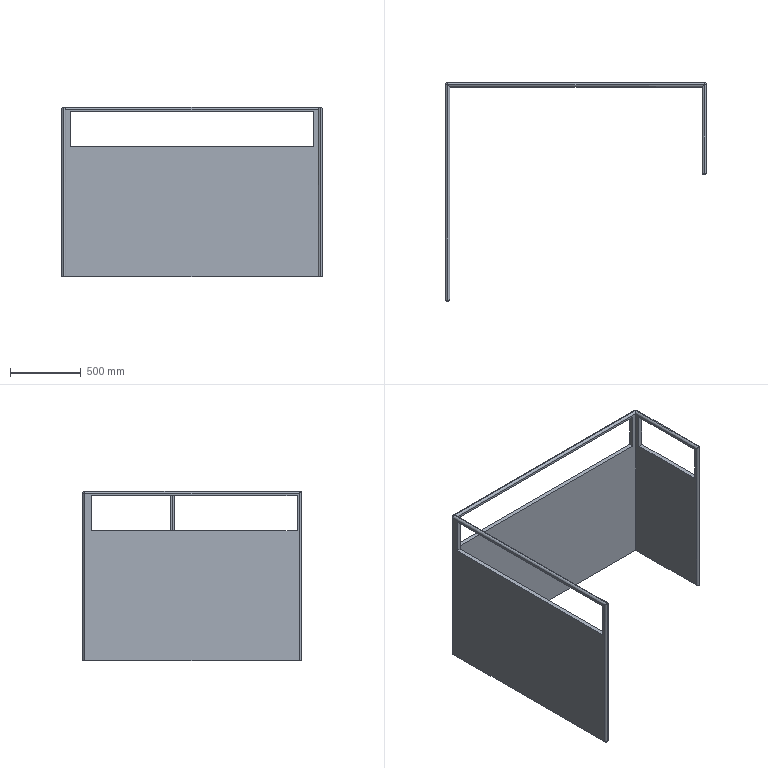Part | SolidWorks | features ICE 3, Extrusion 1, Fillet 1 | 1 solid | 33 faces | box 1850 x 1550 x 1200 mm | volume 114783805 mm3 | plane 19 | cylinder 12 | sphere 2 | commonest cylinder face diameters 30 x12
STEP:
#1=CARTESIAN_POINT('',(30.,30.,1170.));
#2=VERTEX_POINT('',#1);
#3=CARTESIAN_POINT('',(30.,30.,920.));
#4=VERTEX_POINT('',#3);
#5=CARTESIAN_POINT('',(30.,30.,1170.));
#6=DIRECTION('',(0.,0.,-1.));
#7=VECTOR('',#6,1000.);
#8=LINE('',#5,#7);
#9=EDGE_CURVE('',#2,#4,#8,.T.);
#10=ORIENTED_EDGE('',*,*,#9,.F.);
#11=CARTESIAN_POINT('',(30.,1490.,1170.));
#12=VERTEX_POINT('',#11);
#13=CARTESIAN_POINT('',(30.,1490.,1170.));
#14=DIRECTION('',(0.,-1.,0.));
#15=VECTOR('',#14,1000.);
#16=LINE('',#13,#15);
#17=EDGE_CURVE('',#12,#2,#16,.T.);
#18=ORIENTED_EDGE('',*,*,#17,.F.);
#19=CARTESIAN_POINT('',(30.,1490.,920.));
#20=VERTEX_POINT('',#19);
#21=CARTESIAN_POINT('',(30.,1490.,1170.));
#22=DIRECTION('',(0.,0.,1.));
#23=VECTOR('',#22,1000.);
#24=LINE('',#21,#23);
#25=EDGE_CURVE('',#20,#12,#24,.T.);
#26=ORIENTED_EDGE('',*,*,#25,.F.);
#27=CARTESIAN_POINT('',(30.,1490.,920.));
#28=DIRECTION('',(0.,1.,0.));
#29=VECTOR('',#28,1000.);
#30=LINE('',#27,#29);
#31=EDGE_CURVE('',#4,#20,#30,.T.);
#32=ORIENTED_EDGE('',*,*,#31,.F.);
#33=EDGE_LOOP('',(#10,#18,#26,#32));
#34=FACE_BOUND('',#33,.T.);
#35=CARTESIAN_POINT('',(30.,1520.,1185.));
#36=VERTEX_POINT('',#35);
#37=CARTESIAN_POINT('',(30.,15.,1185.));
#38=VERTEX_POINT('',#37);
#39=CARTESIAN_POINT('',(30.,0.,1185.));
#40=DIRECTION('',(0.,-1.,0.));
#41=VECTOR('',#40,1000.);
#42=LINE('',#39,#41);
#43=EDGE_CURVE('',#36,#38,#42,.T.);
#44=ORIENTED_EDGE('',*,*,#43,.T.);
#45=CARTESIAN_POINT('',(30.,15.,0.));
#46=VERTEX_POINT('',#45);
#47=CARTESIAN_POINT('',(30.,15.,1200.));
#48=DIRECTION('',(0.,0.,-1.));
#49=VECTOR('',#48,1000.);
#50=LINE('',#47,#49);
#51=EDGE_CURVE('',#38,#46,#50,.T.);
#52=ORIENTED_EDGE('',*,*,#51,.T.);
#53=CARTESIAN_POINT('',(30.,1520.,0.));
#54=VERTEX_POINT('',#53);
#55=CARTESIAN_POINT('',(30.,0.,0.));
#56=DIRECTION('',(0.,1.,0.));
#57=VECTOR('',#56,1000.);
#58=LINE('',#55,#57);
#59=EDGE_CURVE('',#46,#54,#58,.T.);
#60=ORIENTED_EDGE('',*,*,#59,.T.);
#61=CARTESIAN_POINT('',(30.,1520.,1200.));
#62=DIRECTION('',(0.,0.,-1.));
#63=VECTOR('',#62,1000.);
#64=LINE('',#61,#63);
#65=EDGE_CURVE('',#36,#54,#64,.T.);
#66=ORIENTED_EDGE('',*,*,#65,.F.);
#67=EDGE_LOOP('',(#44,#52,#60,#66));
#68=FACE_OUTER_BOUND('',#67,.T.);
#69=CARTESIAN_POINT('',(30.,0.,1200.));
#70=DIRECTION('',(-1.,0.,0.));
#71=DIRECTION('',(0.,0.,1.));
#72=AXIS2_PLACEMENT_3D('',#69,#70,#71);
#73=PLANE('',#72);
#74=ADVANCED_FACE('',(#34,#68),#73,.F.);
#75=CARTESIAN_POINT('',(60.,1520.,920.));
#76=VERTEX_POINT('',#75);
#77=CARTESIAN_POINT('',(1790.,1520.,920.));
#78=VERTEX_POINT('',#77);
#79=CARTESIAN_POINT('',(60.,1520.,920.));
#80=DIRECTION('',(1.,0.,0.));
#81=VECTOR('',#80,1000.);
#82=LINE('',#79,#81);
#83=EDGE_CURVE('',#76,#78,#82,.T.);
#84=ORIENTED_EDGE('',*,*,#83,.F.);
#85=CARTESIAN_POINT('',(60.,1520.,1170.));
#86=VERTEX_POINT('',#85);
#87=CARTESIAN_POINT('',(60.,1520.,1170.));
#88=DIRECTION('',(0.,0.,-1.));
#89=VECTOR('',#88,1000.);
#90=LINE('',#87,#89);
#91=EDGE_CURVE('',#86,#76,#90,.T.);
#92=ORIENTED_EDGE('',*,*,#91,.F.);
#93=CARTESIAN_POINT('',(1790.,1520.,1170.));
#94=VERTEX_POINT('',#93);
#95=CARTESIAN_POINT('',(60.,1520.,1170.));
#96=DIRECTION('',(-1.,0.,0.));
#97=VECTOR('',#96,1000.);
#98=LINE('',#95,#97);
#99=EDGE_CURVE('',#94,#86,#98,.T.);
#100=ORIENTED_EDGE('',*,*,#99,.F.);
#101=CARTESIAN_POINT('',(1790.,1520.,1170.));
#102=DIRECTION('',(0.,0.,1.));
#103=VECTOR('',#102,1000.);
#104=LINE('',#101,#103);
#105=EDGE_CURVE('',#78,#94,#104,.T.);
#106=ORIENTED_EDGE('',*,*,#105,.F.);
#107=EDGE_LOOP('',(#84,#92,#100,#106));
#108=FACE_BOUND('',#107,.T.);
#109=CARTESIAN_POINT('',(1820.,1520.,1185.));
#110=VERTEX_POINT('',#109);
#111=CARTESIAN_POINT('',(1820.,1520.,0.));
#112=VERTEX_POINT('',#111);
#113=CARTESIAN_POINT('',(1820.,1520.,1200.));
#114=DIRECTION('',(0.,0.,-1.));
#115=VECTOR('',#114,1000.);
#116=LINE('',#113,#115);
#117=EDGE_CURVE('',#110,#112,#116,.T.);
#118=ORIENTED_EDGE('',*,*,#117,.F.);
#119=CARTESIAN_POINT('',(30.,1520.,1185.));
#120=DIRECTION('',(-1.,0.,0.));
#121=VECTOR('',#120,1000.);
#122=LINE('',#119,#121);
#123=EDGE_CURVE('',#110,#36,#122,.T.);
#124=ORIENTED_EDGE('',*,*,#123,.T.);
#125=ORIENTED_EDGE('',*,*,#65,.T.);
#126=CARTESIAN_POINT('',(30.,1520.,0.));
#127=DIRECTION('',(1.,0.,0.));
#128=VECTOR('',#127,1000.);
#129=LINE('',#126,#128);
#130=EDGE_CURVE('',#54,#112,#129,.T.);
#131=ORIENTED_EDGE('',*,*,#130,.T.);
#132=EDGE_LOOP('',(#118,#124,#125,#131));
#133=FACE_OUTER_BOUND('',#132,.T.);
#134=CARTESIAN_POINT('',(30.,1520.,1200.));
#135=DIRECTION('',(0.,1.,0.));
#136=DIRECTION('',(0.,0.,1.));
#137=AXIS2_PLACEMENT_3D('',#134,#135,#136);
#138=PLANE('',#137);
#139=ADVANCED_FACE('',(#108,#133),#138,.F.);
#140=CARTESIAN_POINT('',(1820.,930.,920.));
#141=VERTEX_POINT('',#140);
#142=CARTESIAN_POINT('',(1820.,930.,1170.));
#143=VERTEX_POINT('',#142);
#144=CARTESIAN_POINT('',(1820.,930.,920.));
#145=DIRECTION('',(0.,0.,1.));
#146=VECTOR('',#145,1000.);
#147=LINE('',#144,#146);
#148=EDGE_CURVE('',#141,#143,#147,.T.);
#149=ORIENTED_EDGE('',*,*,#148,.F.);
#150=CARTESIAN_POINT('',(1820.,1490.,920.));
#151=VERTEX_POINT('',#150);
#152=CARTESIAN_POINT('',(1820.,1490.,920.));
#153=DIRECTION('',(0.,-1.,0.));
#154=VECTOR('',#153,1000.);
#155=LINE('',#152,#154);
#156=EDGE_CURVE('',#151,#141,#155,.T.);
#157=ORIENTED_EDGE('',*,*,#156,.F.);
#158=CARTESIAN_POINT('',(1820.,1490.,1170.));
#159=VERTEX_POINT('',#158);
#160=CARTESIAN_POINT('',(1820.,1490.,920.));
#161=DIRECTION('',(0.,0.,-1.));
#162=VECTOR('',#161,1000.);
#163=LINE('',#160,#162);
#164=EDGE_CURVE('',#159,#151,#163,.T.);
#165=ORIENTED_EDGE('',*,*,#164,.F.);
#166=CARTESIAN_POINT('',(1820.,1490.,1170.));
#167=DIRECTION('',(0.,1.,0.));
#168=VECTOR('',#167,1000.);
#169=LINE('',#166,#168);
#170=EDGE_CURVE('',#143,#159,#169,.T.);
#171=ORIENTED_EDGE('',*,*,#170,.F.);
#172=EDGE_LOOP('',(#149,#157,#165,#171));
#173=FACE_BOUND('',#172,.T.);
#174=CARTESIAN_POINT('',(1820.,915.,0.));
#175=VERTEX_POINT('',#174);
#176=CARTESIAN_POINT('',(1820.,1520.,0.));
#177=DIRECTION('',(0.,-1.,0.));
#178=VECTOR('',#177,1000.);
#179=LINE('',#176,#178);
#180=EDGE_CURVE('',#112,#175,#179,.T.);
#181=ORIENTED_EDGE('',*,*,#180,.T.);
#182=CARTESIAN_POINT('',(1820.,915.,1185.));
#183=VERTEX_POINT('',#182);
#184=CARTESIAN_POINT('',(1820.,915.,1200.));
#185=DIRECTION('',(0.,0.,1.));
#186=VECTOR('',#185,1000.);
#187=LINE('',#184,#186);
#188=EDGE_CURVE('',#175,#183,#187,.T.);
#189=ORIENTED_EDGE('',*,*,#188,.T.);
#190=CARTESIAN_POINT('',(1820.,1520.,1185.));
#191=DIRECTION('',(0.,1.,0.));
#192=VECTOR('',#191,1000.);
#193=LINE('',#190,#192);
#194=EDGE_CURVE('',#183,#110,#193,.T.);
#195=ORIENTED_EDGE('',*,*,#194,.T.);
#196=ORIENTED_EDGE('',*,*,#117,.T.);
#197=EDGE_LOOP('',(#181,#189,#195,#196));
#198=FACE_OUTER_BOUND('',#197,.T.);
#199=CARTESIAN_POINT('',(1820.,1520.,1200.));
#200=DIRECTION('',(1.,0.,0.));
#201=DIRECTION('',(0.,0.,-1.));
#202=AXIS2_PLACEMENT_3D('',#199,#200,#201);
#203=PLANE('',#202);
#204=ADVANCED_FACE('',(#173,#198),#203,.F.);
#205=CARTESIAN_POINT('',(1850.,1535.,0.));
#206=VERTEX_POINT('',#205);
#207=CARTESIAN_POINT('',(1850.,915.,0.));
#208=VERTEX_POINT('',#207);
#209=CARTESIAN_POINT('',(1850.,1550.,0.));
#210=DIRECTION('',(0.,-1.,0.));
#211=VECTOR('',#210,1000.);
#212=LINE('',#209,#211);
#213=EDGE_CURVE('',#206,#208,#212,.T.);
#214=ORIENTED_EDGE('',*,*,#213,.F.);
#215=CARTESIAN_POINT('',(1850.,1535.,1185.));
#216=VERTEX_POINT('',#215);
#217=CARTESIAN_POINT('',(1850.,1535.,1200.));
#218=DIRECTION('',(0.,0.,1.));
#219=VECTOR('',#218,1000.);
#220=LINE('',#217,#219);
#221=EDGE_CURVE('',#206,#216,#220,.T.);
#222=ORIENTED_EDGE('',*,*,#221,.T.);
#223=CARTESIAN_POINT('',(1850.,915.,1185.));
#224=VERTEX_POINT('',#223);
#225=CARTESIAN_POINT('',(1850.,900.,1185.));
#226=DIRECTION('',(0.,-1.,0.));
#227=VECTOR('',#226,1000.);
#228=LINE('',#225,#227);
#229=EDGE_CURVE('',#216,#224,#228,.T.);
#230=ORIENTED_EDGE('',*,*,#229,.T.);
#231=CARTESIAN_POINT('',(1850.,915.,1200.));
#232=DIRECTION('',(0.,0.,-1.));
#233=VECTOR('',#232,1000.);
#234=LINE('',#231,#233);
#235=EDGE_CURVE('',#224,#208,#234,.T.);
#236=ORIENTED_EDGE('',*,*,#235,.T.);
#237=EDGE_LOOP('',(#214,#222,#230,#236));
#238=FACE_OUTER_BOUND('',#237,.T.);
#239=CARTESIAN_POINT('',(1850.,1490.,920.));
#240=VERTEX_POINT('',#239);
#241=CARTESIAN_POINT('',(1850.,930.,920.));
#242=VERTEX_POINT('',#241);
#243=CARTESIAN_POINT('',(1850.,1490.,920.));
#244=DIRECTION('',(0.,-1.,0.));
#245=VECTOR('',#244,1000.);
#246=LINE('',#243,#245);
#247=EDGE_CURVE('',#240,#242,#246,.T.);
#248=ORIENTED_EDGE('',*,*,#247,.T.);
#249=CARTESIAN_POINT('',(1850.,930.,1170.));
#250=VERTEX_POINT('',#249);
#251=CARTESIAN_POINT('',(1850.,930.,920.));
#252=DIRECTION('',(0.,0.,1.));
#253=VECTOR('',#252,1000.);
#254=LINE('',#251,#253);
#255=EDGE_CURVE('',#242,#250,#254,.T.);
#256=ORIENTED_EDGE('',*,*,#255,.T.);
#257=CARTESIAN_POINT('',(1850.,1490.,1170.));
#258=VERTEX_POINT('',#257);
#259=CARTESIAN_POINT('',(1850.,1490.,1170.));
#260=DIRECTION('',(0.,1.,0.));
#261=VECTOR('',#260,1000.);
#262=LINE('',#259,#261);
#263=EDGE_CURVE('',#250,#258,#262,.T.);
#264=ORIENTED_EDGE('',*,*,#263,.T.);
#265=CARTESIAN_POINT('',(1850.,1490.,920.));
#266=DIRECTION('',(0.,0.,-1.));
#267=VECTOR('',#266,1000.);
#268=LINE('',#265,#267);
#269=EDGE_CURVE('',#258,#240,#268,.T.);
#270=ORIENTED_EDGE('',*,*,#269,.T.);
#271=EDGE_LOOP('',(#248,#256,#264,#270));
#272=FACE_BOUND('',#271,.T.);
#273=CARTESIAN_POINT('',(1850.,1550.,1200.));
#274=DIRECTION('',(1.,0.,0.));
#275=DIRECTION('',(0.,1.,0.));
#276=AXIS2_PLACEMENT_3D('',#273,#274,#275);
#277=PLANE('',#276);
#278=ADVANCED_FACE('',(#238,#272),#277,.T.);
#279=CARTESIAN_POINT('',(60.,1550.,1170.));
#280=VERTEX_POINT('',#279);
#281=CARTESIAN_POINT('',(60.,1550.,920.));
#282=VERTEX_POINT('',#281);
#283=CARTESIAN_POINT('',(60.,1550.,1170.));
#284=DIRECTION('',(0.,0.,-1.));
#285=VECTOR('',#284,1000.);
#286=LINE('',#283,#285);
#287=EDGE_CURVE('',#280,#282,#286,.T.);
#288=ORIENTED_EDGE('',*,*,#287,.T.);
#289=CARTESIAN_POINT('',(1790.,1550.,920.));
#290=VERTEX_POINT('',#289);
#291=CARTESIAN_POINT('',(60.,1550.,920.));
#292=DIRECTION('',(1.,0.,0.));
#293=VECTOR('',#292,1000.);
#294=LINE('',#291,#293);
#295=EDGE_CURVE('',#282,#290,#294,.T.);
#296=ORIENTED_EDGE('',*,*,#295,.T.);
#297=CARTESIAN_POINT('',(1790.,1550.,1170.));
#298=VERTEX_POINT('',#297);
#299=CARTESIAN_POINT('',(1790.,1550.,1170.));
#300=DIRECTION('',(0.,0.,1.));
#301=VECTOR('',#300,1000.);
#302=LINE('',#299,#301);
#303=EDGE_CURVE('',#290,#298,#302,.T.);
#304=ORIENTED_EDGE('',*,*,#303,.T.);
#305=CARTESIAN_POINT('',(60.,1550.,1170.));
#306=DIRECTION('',(-1.,0.,0.));
#307=VECTOR('',#306,1000.);
#308=LINE('',#305,#307);
#309=EDGE_CURVE('',#298,#280,#308,.T.);
#310=ORIENTED_EDGE('',*,*,#309,.T.);
#311=EDGE_LOOP('',(#288,#296,#304,#310));
#312=FACE_BOUND('',#311,.T.);
#313=CARTESIAN_POINT('',(15.,1550.,1185.));
#314=VERTEX_POINT('',#313);
#315=CARTESIAN_POINT('',(1835.,1550.,1185.));
#316=VERTEX_POINT('',#315);
#317=CARTESIAN_POINT('',(1850.,1550.,1185.));
#318=DIRECTION('',(1.,0.,0.));
#319=VECTOR('',#318,1000.);
#320=LINE('',#317,#319);
#321=EDGE_CURVE('',#314,#316,#320,.T.);
#322=ORIENTED_EDGE('',*,*,#321,.T.);
#323=CARTESIAN_POINT('',(1835.,1550.,0.));
#324=VERTEX_POINT('',#323);
#325=CARTESIAN_POINT('',(1835.,1550.,1200.));
#326=DIRECTION('',(0.,0.,-1.));
#327=VECTOR('',#326,1000.);
#328=LINE('',#325,#327);
#329=EDGE_CURVE('',#316,#324,#328,.T.);
#330=ORIENTED_EDGE('',*,*,#329,.T.);
#331=CARTESIAN_POINT('',(15.,1550.,0.));
#332=VERTEX_POINT('',#331);
#333=CARTESIAN_POINT('',(0.,1550.,0.));
#334=DIRECTION('',(1.,0.,0.));
#335=VECTOR('',#334,1000.);
#336=LINE('',#333,#335);
#337=EDGE_CURVE('',#332,#324,#336,.T.);
#338=ORIENTED_EDGE('',*,*,#337,.F.);
#339=CARTESIAN_POINT('',(15.,1550.,1200.));
#340=DIRECTION('',(0.,0.,1.));
#341=VECTOR('',#340,1000.);
#342=LINE('',#339,#341);
#343=EDGE_CURVE('',#332,#314,#342,.T.);
#344=ORIENTED_EDGE('',*,*,#343,.T.);
#345=EDGE_LOOP('',(#322,#330,#338,#344));
#346=FACE_OUTER_BOUND('',#345,.T.);
#347=CARTESIAN_POINT('',(0.,1550.,1200.));
#348=DIRECTION('',(0.,1.,0.));
#349=DIRECTION('',(0.,0.,1.));
#350=AXIS2_PLACEMENT_3D('',#347,#348,#349);
#351=PLANE('',#350);
#352=ADVANCED_FACE('',(#312,#346),#351,.T.);
#353=CARTESIAN_POINT('',(0.,1490.,1170.));
#354=VERTEX_POINT('',#353);
#355=CARTESIAN_POINT('',(0.,30.,1170.));
#356=VERTEX_POINT('',#355);
#357=CARTESIAN_POINT('',(0.,1490.,1170.));
#358=DIRECTION('',(0.,-1.,0.));
#359=VECTOR('',#358,1000.);
#360=LINE('',#357,#359);
#361=EDGE_CURVE('',#354,#356,#360,.T.);
#362=ORIENTED_EDGE('',*,*,#361,.T.);
#363=CARTESIAN_POINT('',(0.,30.,920.));
#364=VERTEX_POINT('',#363);
#365=CARTESIAN_POINT('',(0.,30.,1170.));
#366=DIRECTION('',(0.,0.,-1.));
#367=VECTOR('',#366,1000.);
#368=LINE('',#365,#367);
#369=EDGE_CURVE('',#356,#364,#368,.T.);
#370=ORIENTED_EDGE('',*,*,#369,.T.);
#371=CARTESIAN_POINT('',(0.,1490.,920.));
#372=VERTEX_POINT('',#371);
#373=CARTESIAN_POINT('',(0.,1490.,920.));
#374=DIRECTION('',(0.,1.,0.));
#375=VECTOR('',#374,1000.);
#376=LINE('',#373,#375);
#377=EDGE_CURVE('',#364,#372,#376,.T.);
#378=ORIENTED_EDGE('',*,*,#377,.T.);
#379=CARTESIAN_POINT('',(0.,1490.,1170.));
#380=DIRECTION('',(0.,0.,1.));
#381=VECTOR('',#380,1000.);
#382=LINE('',#379,#381);
#383=EDGE_CURVE('',#372,#354,#382,.T.);
#384=ORIENTED_EDGE('',*,*,#383,.T.);
#385=EDGE_LOOP('',(#362,#370,#378,#384));
#386=FACE_BOUND('',#385,.T.);
#387=CARTESIAN_POINT('',(0.,15.,1185.));
#388=VERTEX_POINT('',#387);
#389=CARTESIAN_POINT('',(0.,1535.,1185.));
#390=VERTEX_POINT('',#389);
#391=CARTESIAN_POINT('',(0.,1550.,1185.));
#392=DIRECTION('',(0.,1.,0.));
#393=VECTOR('',#392,1000.);
#394=LINE('',#391,#393);
#395=EDGE_CURVE('',#388,#390,#394,.T.);
#396=ORIENTED_EDGE('',*,*,#395,.T.);
#397=CARTESIAN_POINT('',(0.,1535.,0.));
#398=VERTEX_POINT('',#397);
#399=CARTESIAN_POINT('',(0.,1535.,1200.));
#400=DIRECTION('',(0.,0.,-1.));
#401=VECTOR('',#400,1000.);
#402=LINE('',#399,#401);
#403=EDGE_CURVE('',#390,#398,#402,.T.);
#404=ORIENTED_EDGE('',*,*,#403,.T.);
#405=CARTESIAN_POINT('',(0.,15.,0.));
#406=VERTEX_POINT('',#405);
#407=CARTESIAN_POINT('',(0.,0.,0.));
#408=DIRECTION('',(0.,1.,0.));
#409=VECTOR('',#408,1000.);
#410=LINE('',#407,#409);
#411=EDGE_CURVE('',#406,#398,#410,.T.);
#412=ORIENTED_EDGE('',*,*,#411,.F.);
#413=CARTESIAN_POINT('',(0.,15.,1200.));
#414=DIRECTION('',(0.,0.,1.));
#415=VECTOR('',#414,1000.);
#416=LINE('',#413,#415);
#417=EDGE_CURVE('',#406,#388,#416,.T.);
#418=ORIENTED_EDGE('',*,*,#417,.T.);
#419=EDGE_LOOP('',(#396,#404,#412,#418));
#420=FACE_OUTER_BOUND('',#419,.T.);
#421=CARTESIAN_POINT('',(0.,0.,1200.));
#422=DIRECTION('',(-1.,0.,0.));
#423=DIRECTION('',(0.,0.,1.));
#424=AXIS2_PLACEMENT_3D('',#421,#422,#423);
#425=PLANE('',#424);
#426=ADVANCED_FACE('',(#386,#420),#425,.T.);
#427=ORIENTED_EDGE('',*,*,#337,.T.);
#428=CARTESIAN_POINT('',(1835.,1535.,0.));
#429=DIRECTION('',(0.,0.,-1.));
#430=DIRECTION('',(-1.,0.,0.));
#431=AXIS2_PLACEMENT_3D('',#428,#429,#430);
#432=CIRCLE('',#431,15.);
#433=EDGE_CURVE('',#324,#206,#432,.T.);
#434=ORIENTED_EDGE('',*,*,#433,.T.);
#435=ORIENTED_EDGE('',*,*,#213,.T.);
#436=CARTESIAN_POINT('',(1835.,900.,0.));
#437=VERTEX_POINT('',#436);
#438=CARTESIAN_POINT('',(1835.,915.,0.));
#439=DIRECTION('',(0.,0.,-1.));
#440=DIRECTION('',(-1.,0.,0.));
#441=AXIS2_PLACEMENT_3D('',#438,#439,#440);
#442=CIRCLE('',#441,15.);
#443=EDGE_CURVE('',#208,#437,#442,.T.);
#444=ORIENTED_EDGE('',*,*,#443,.T.);
#445=CARTESIAN_POINT('',(1835.,915.,0.));
#446=DIRECTION('',(0.,0.,-1.));
#447=DIRECTION('',(-1.,0.,0.));
#448=AXIS2_PLACEMENT_3D('',#445,#446,#447);
#449=CIRCLE('',#448,15.);
#450=EDGE_CURVE('',#437,#175,#449,.T.);
#451=ORIENTED_EDGE('',*,*,#450,.T.);
#452=ORIENTED_EDGE('',*,*,#180,.F.);
#453=ORIENTED_EDGE('',*,*,#130,.F.);
#454=ORIENTED_EDGE('',*,*,#59,.F.);
#455=CARTESIAN_POINT('',(15.,0.,0.));
#456=VERTEX_POINT('',#455);
#457=CARTESIAN_POINT('',(15.,15.,0.));
#458=DIRECTION('',(0.,0.,-1.));
#459=DIRECTION('',(-1.,0.,0.));
#460=AXIS2_PLACEMENT_3D('',#457,#458,#459);
#461=CIRCLE('',#460,15.);
#462=EDGE_CURVE('',#46,#456,#461,.T.);
#463=ORIENTED_EDGE('',*,*,#462,.T.);
#464=CARTESIAN_POINT('',(15.,15.,0.));
#465=DIRECTION('',(0.,0.,-1.));
#466=DIRECTION('',(-1.,0.,0.));
#467=AXIS2_PLACEMENT_3D('',#464,#465,#466);
#468=CIRCLE('',#467,15.);
#469=EDGE_CURVE('',#456,#406,#468,.T.);
#470=ORIENTED_EDGE('',*,*,#469,.T.);
#471=ORIENTED_EDGE('',*,*,#411,.T.);
#472=CARTESIAN_POINT('',(15.,1535.,0.));
#473=DIRECTION('',(0.,0.,-1.));
#474=DIRECTION('',(-1.,0.,0.));
#475=AXIS2_PLACEMENT_3D('',#472,#473,#474);
#476=CIRCLE('',#475,15.);
#477=EDGE_CURVE('',#398,#332,#476,.T.);
#478=ORIENTED_EDGE('',*,*,#477,.T.);
#479=EDGE_LOOP('',(#427,#434,#435,#444,#451,#452,#453,#454,#463,#470,#471,#478));
#480=FACE_OUTER_BOUND('',#479,.T.);
#481=CARTESIAN_POINT('',(30.,1520.,0.));
#482=DIRECTION('',(0.,0.,-1.));
#483=DIRECTION('',(-1.,0.,0.));
#484=AXIS2_PLACEMENT_3D('',#481,#482,#483);
#485=PLANE('',#484);
#486=ADVANCED_FACE('',(#480),#485,.T.);
#487=ORIENTED_EDGE('',*,*,#91,.T.);
#488=CARTESIAN_POINT('',(60.,1550.,920.));
#489=DIRECTION('',(0.,-1.,0.));
#490=VECTOR('',#489,1000.);
#491=LINE('',#488,#490);
#492=EDGE_CURVE('',#282,#76,#491,.T.);
#493=ORIENTED_EDGE('',*,*,#492,.F.);
#494=ORIENTED_EDGE('',*,*,#287,.F.);
#495=CARTESIAN_POINT('',(60.,1550.,1170.));
#496=DIRECTION('',(0.,-1.,0.));
#497=VECTOR('',#496,1000.);
#498=LINE('',#495,#497);
#499=EDGE_CURVE('',#280,#86,#498,.T.);
#500=ORIENTED_EDGE('',*,*,#499,.T.);
#501=EDGE_LOOP('',(#487,#493,#494,#500));
#502=FACE_OUTER_BOUND('',#501,.T.);
#503=CARTESIAN_POINT('',(60.,1550.,1170.));
#504=DIRECTION('',(-1.,0.,0.));
#505=DIRECTION('',(0.,0.,1.));
#506=AXIS2_PLACEMENT_3D('',#503,#504,#505);
#507=PLANE('',#506);
#508=ADVANCED_FACE('',(#502),#507,.F.);
#509=ORIENTED_EDGE('',*,*,#99,.T.);
#510=ORIENTED_EDGE('',*,*,#499,.F.);
#511=ORIENTED_EDGE('',*,*,#309,.F.);
#512=CARTESIAN_POINT('',(1790.,1550.,1170.));
#513=DIRECTION('',(0.,-1.,0.));
#514=VECTOR('',#513,1000.);
#515=LINE('',#512,#514);
#516=EDGE_CURVE('',#298,#94,#515,.T.);
#517=ORIENTED_EDGE('',*,*,#516,.T.);
#518=EDGE_LOOP('',(#509,#510,#511,#517));
#519=FACE_OUTER_BOUND('',#518,.T.);
#520=CARTESIAN_POINT('',(60.,1550.,1170.));
#521=DIRECTION('',(0.,0.,1.));
#522=DIRECTION('',(1.,0.,0.));
#523=AXIS2_PLACEMENT_3D('',#520,#521,#522);
#524=PLANE('',#523);
#525=ADVANCED_FACE('',(#519),#524,.F.);
#526=ORIENTED_EDGE('',*,*,#105,.T.);
#527=ORIENTED_EDGE('',*,*,#516,.F.);
#528=ORIENTED_EDGE('',*,*,#303,.F.);
#529=CARTESIAN_POINT('',(1790.,1550.,920.));
#530=DIRECTION('',(0.,-1.,0.));
#531=VECTOR('',#530,1000.);
#532=LINE('',#529,#531);
#533=EDGE_CURVE('',#290,#78,#532,.T.);
#534=ORIENTED_EDGE('',*,*,#533,.T.);
#535=EDGE_LOOP('',(#526,#527,#528,#534));
#536=FACE_OUTER_BOUND('',#535,.T.);
#537=CARTESIAN_POINT('',(1790.,1550.,1170.));
#538=DIRECTION('',(1.,0.,0.));
#539=DIRECTION('',(0.,0.,-1.));
#540=AXIS2_PLACEMENT_3D('',#537,#538,#539);
#541=PLANE('',#540);
#542=ADVANCED_FACE('',(#536),#541,.F.);
#543=ORIENTED_EDGE('',*,*,#83,.T.);
#544=ORIENTED_EDGE('',*,*,#533,.F.);
#545=ORIENTED_EDGE('',*,*,#295,.F.);
#546=ORIENTED_EDGE('',*,*,#492,.T.);
#547=EDGE_LOOP('',(#543,#544,#545,#546));
#548=FACE_OUTER_BOUND('',#547,.T.);
#549=CARTESIAN_POINT('',(60.,1550.,920.));
#550=DIRECTION('',(0.,0.,-1.));
#551=DIRECTION('',(-1.,0.,0.));
#552=AXIS2_PLACEMENT_3D('',#549,#550,#551);
#553=PLANE('',#552);
#554=ADVANCED_FACE('',(#548),#553,.F.);
#555=ORIENTED_EDGE('',*,*,#17,.T.);
#556=CARTESIAN_POINT('',(0.,30.,1170.));
#557=DIRECTION('',(1.,0.,0.));
#558=VECTOR('',#557,1000.);
#559=LINE('',#556,#558);
#560=EDGE_CURVE('',#356,#2,#559,.T.);
#561=ORIENTED_EDGE('',*,*,#560,.F.);
#562=ORIENTED_EDGE('',*,*,#361,.F.);
#563=CARTESIAN_POINT('',(0.,1490.,1170.));
#564=DIRECTION('',(1.,0.,0.));
#565=VECTOR('',#564,1000.);
#566=LINE('',#563,#565);
#567=EDGE_CURVE('',#354,#12,#566,.T.);
#568=ORIENTED_EDGE('',*,*,#567,.T.);
#569=EDGE_LOOP('',(#555,#561,#562,#568));
#570=FACE_OUTER_BOUND('',#569,.T.);
#571=CARTESIAN_POINT('',(0.,1490.,1170.));
#572=DIRECTION('',(0.,0.,1.));
#573=DIRECTION('',(0.,-1.,0.));
#574=AXIS2_PLACEMENT_3D('',#571,#572,#573);
#575=PLANE('',#574);
#576=ADVANCED_FACE('',(#570),#575,.F.);
#577=ORIENTED_EDGE('',*,*,#25,.T.);
#578=ORIENTED_EDGE('',*,*,#567,.F.);
#579=ORIENTED_EDGE('',*,*,#383,.F.);
#580=CARTESIAN_POINT('',(0.,1490.,920.));
#581=DIRECTION('',(1.,0.,0.));
#582=VECTOR('',#581,1000.);
#583=LINE('',#580,#582);
#584=EDGE_CURVE('',#372,#20,#583,.T.);
#585=ORIENTED_EDGE('',*,*,#584,.T.);
#586=EDGE_LOOP('',(#577,#578,#579,#585));
#587=FACE_OUTER_BOUND('',#586,.T.);
#588=CARTESIAN_POINT('',(0.,1490.,1170.));
#589=DIRECTION('',(0.,1.,0.));
#590=DIRECTION('',(0.,0.,1.));
#591=AXIS2_PLACEMENT_3D('',#588,#589,#590);
#592=PLANE('',#591);
#593=ADVANCED_FACE('',(#587),#592,.F.);
#594=ORIENTED_EDGE('',*,*,#31,.T.);
#595=ORIENTED_EDGE('',*,*,#584,.F.);
#596=ORIENTED_EDGE('',*,*,#377,.F.);
#597=CARTESIAN_POINT('',(0.,30.,920.));
#598=DIRECTION('',(1.,0.,0.));
#599=VECTOR('',#598,1000.);
#600=LINE('',#597,#599);
#601=EDGE_CURVE('',#364,#4,#600,.T.);
#602=ORIENTED_EDGE('',*,*,#601,.T.);
#603=EDGE_LOOP('',(#594,#595,#596,#602));
#604=FACE_OUTER_BOUND('',#603,.T.);
#605=CARTESIAN_POINT('',(0.,1490.,920.));
#606=DIRECTION('',(0.,0.,-1.));
#607=DIRECTION('',(0.,1.,0.));
#608=AXIS2_PLACEMENT_3D('',#605,#606,#607);
#609=PLANE('',#608);
#610=ADVANCED_FACE('',(#604),#609,.F.);
#611=ORIENTED_EDGE('',*,*,#9,.T.);
#612=ORIENTED_EDGE('',*,*,#601,.F.);
#613=ORIENTED_EDGE('',*,*,#369,.F.);
#614=ORIENTED_EDGE('',*,*,#560,.T.);
#615=EDGE_LOOP('',(#611,#612,#613,#614));
#616=FACE_OUTER_BOUND('',#615,.T.);
#617=CARTESIAN_POINT('',(0.,30.,1170.));
#618=DIRECTION('',(0.,-1.,0.));
#619=DIRECTION('',(0.,0.,-1.));
#620=AXIS2_PLACEMENT_3D('',#617,#618,#619);
#621=PLANE('',#620);
#622=ADVANCED_FACE('',(#616),#621,.F.);
#623=ORIENTED_EDGE('',*,*,#156,.T.);
#624=CARTESIAN_POINT('',(1850.,930.,920.));
#625=DIRECTION('',(-1.,0.,0.));
#626=VECTOR('',#625,1000.);
#627=LINE('',#624,#626);
#628=EDGE_CURVE('',#242,#141,#627,.T.);
#629=ORIENTED_EDGE('',*,*,#628,.F.);
#630=ORIENTED_EDGE('',*,*,#247,.F.);
#631=CARTESIAN_POINT('',(1850.,1490.,920.));
#632=DIRECTION('',(-1.,0.,0.));
#633=VECTOR('',#632,1000.);
#634=LINE('',#631,#633);
#635=EDGE_CURVE('',#240,#151,#634,.T.);
#636=ORIENTED_EDGE('',*,*,#635,.T.);
#637=EDGE_LOOP('',(#623,#629,#630,#636));
#638=FACE_OUTER_BOUND('',#637,.T.);
#639=CARTESIAN_POINT('',(1850.,1490.,920.));
#640=DIRECTION('',(0.,0.,-1.));
#641=DIRECTION('',(0.,1.,0.));
#642=AXIS2_PLACEMENT_3D('',#639,#640,#641);
#643=PLANE('',#642);
#644=ADVANCED_FACE('',(#638),#643,.F.);
#645=ORIENTED_EDGE('',*,*,#164,.T.);
#646=ORIENTED_EDGE('',*,*,#635,.F.);
#647=ORIENTED_EDGE('',*,*,#269,.F.);
#648=CARTESIAN_POINT('',(1850.,1490.,1170.));
#649=DIRECTION('',(-1.,0.,0.));
#650=VECTOR('',#649,1000.);
#651=LINE('',#648,#650);
#652=EDGE_CURVE('',#258,#159,#651,.T.);
#653=ORIENTED_EDGE('',*,*,#652,.T.);
#654=EDGE_LOOP('',(#645,#646,#647,#653));
#655=FACE_OUTER_BOUND('',#654,.T.);
#656=CARTESIAN_POINT('',(1850.,1490.,920.));
#657=DIRECTION('',(0.,1.,0.));
#658=DIRECTION('',(-1.,0.,0.));
#659=AXIS2_PLACEMENT_3D('',#656,#657,#658);
#660=PLANE('',#659);
#661=ADVANCED_FACE('',(#655),#660,.F.);
#662=ORIENTED_EDGE('',*,*,#170,.T.);
#663=ORIENTED_EDGE('',*,*,#652,.F.);
#664=ORIENTED_EDGE('',*,*,#263,.F.);
#665=CARTESIAN_POINT('',(1850.,930.,1170.));
#666=DIRECTION('',(-1.,0.,0.));
#667=VECTOR('',#666,1000.);
#668=LINE('',#665,#667);
#669=EDGE_CURVE('',#250,#143,#668,.T.);
#670=ORIENTED_EDGE('',*,*,#669,.T.);
#671=EDGE_LOOP('',(#662,#663,#664,#670));
#672=FACE_OUTER_BOUND('',#671,.T.);
#673=CARTESIAN_POINT('',(1850.,1490.,1170.));
#674=DIRECTION('',(0.,0.,1.));
#675=DIRECTION('',(1.,0.,0.));
#676=AXIS2_PLACEMENT_3D('',#673,#674,#675);
#677=PLANE('',#676);
#678=ADVANCED_FACE('',(#672),#677,.F.);
#679=ORIENTED_EDGE('',*,*,#148,.T.);
#680=ORIENTED_EDGE('',*,*,#669,.F.);
#681=ORIENTED_EDGE('',*,*,#255,.F.);
#682=ORIENTED_EDGE('',*,*,#628,.T.);
#683=EDGE_LOOP('',(#679,#680,#681,#682));
#684=FACE_OUTER_BOUND('',#683,.T.);
#685=CARTESIAN_POINT('',(1850.,930.,920.));
#686=DIRECTION('',(0.,-1.,0.));
#687=DIRECTION('',(1.,0.,0.));
#688=AXIS2_PLACEMENT_3D('',#685,#686,#687);
#689=PLANE('',#688);
#690=ADVANCED_FACE('',(#684),#689,.F.);
#691=CARTESIAN_POINT('',(15.,0.,1200.));
#692=VERTEX_POINT('',#691);
#693=CARTESIAN_POINT('',(15.,0.,1200.));
#694=DIRECTION('',(0.,0.,1.));
#695=VECTOR('',#694,1000.);
#696=LINE('',#693,#695);
#697=EDGE_CURVE('',#456,#692,#696,.T.);
#698=ORIENTED_EDGE('',*,*,#697,.F.);
#699=ORIENTED_EDGE('',*,*,#462,.F.);
#700=ORIENTED_EDGE('',*,*,#51,.F.);
#701=CARTESIAN_POINT('',(15.,0.,1200.));
#702=CARTESIAN_POINT('',(23.787,0.,1200.));
#703=CARTESIAN_POINT('',(30.,6.213,1193.787));
#704=CARTESIAN_POINT('',(30.,15.,1185.));
#705=(BOUNDED_CURVE()B_SPLINE_CURVE(3,(#701,#702,#703,#704),.UNSPECIFIED.,.F.,.F.)B_SPLINE_CURVE_WITH_KNOTS((4,4),(3.142,4.712),.UNSPECIFIED.)CURVE()GEOMETRIC_REPRESENTATION_ITEM()RATIONAL_B_SPLINE_CURVE((1.,0.8047,0.8047,1.))REPRESENTATION_ITEM(''));
#706=EDGE_CURVE('',#692,#38,#705,.T.);
#707=ORIENTED_EDGE('',*,*,#706,.F.);
#708=EDGE_LOOP('',(#698,#699,#700,#707));
#709=FACE_OUTER_BOUND('',#708,.T.);
#710=CARTESIAN_POINT('',(15.,15.,1200.));
#711=DIRECTION('',(0.,0.,-1.));
#712=DIRECTION('',(-1.,0.,0.));
#713=AXIS2_PLACEMENT_3D('',#710,#711,#712);
#714=CYLINDRICAL_SURFACE('',#713,15.);
#715=ADVANCED_FACE('',(#709),#714,.T.);
#716=ORIENTED_EDGE('',*,*,#469,.F.);
#717=ORIENTED_EDGE('',*,*,#697,.T.);
#718=CARTESIAN_POINT('',(0.,15.,1185.));
#719=CARTESIAN_POINT('',(0.,6.213,1193.787));
#720=CARTESIAN_POINT('',(6.213,0.,1200.));
#721=CARTESIAN_POINT('',(15.,0.,1200.));
#722=(BOUNDED_CURVE()B_SPLINE_CURVE(3,(#718,#719,#720,#721),.UNSPECIFIED.,.F.,.F.)B_SPLINE_CURVE_WITH_KNOTS((4,4),(4.712,6.283),.UNSPECIFIED.)CURVE()GEOMETRIC_REPRESENTATION_ITEM()RATIONAL_B_SPLINE_CURVE((1.,0.8047,0.8047,1.))REPRESENTATION_ITEM(''));
#723=EDGE_CURVE('',#388,#692,#722,.T.);
#724=ORIENTED_EDGE('',*,*,#723,.F.);
#725=ORIENTED_EDGE('',*,*,#417,.F.);
#726=EDGE_LOOP('',(#716,#717,#724,#725));
#727=FACE_OUTER_BOUND('',#726,.T.);
#728=CARTESIAN_POINT('',(15.,15.,1200.));
#729=DIRECTION('',(0.,0.,1.));
#730=DIRECTION('',(1.,0.,0.));
#731=AXIS2_PLACEMENT_3D('',#728,#729,#730);
#732=CYLINDRICAL_SURFACE('',#731,15.);
#733=ADVANCED_FACE('',(#727),#732,.T.);
#734=ORIENTED_EDGE('',*,*,#188,.F.);
#735=ORIENTED_EDGE('',*,*,#450,.F.);
#736=CARTESIAN_POINT('',(1835.,900.,1200.));
#737=VERTEX_POINT('',#736);
#738=CARTESIAN_POINT('',(1835.,900.,0.));
#739=DIRECTION('',(0.,0.,-1.));
#740=VECTOR('',#739,1000.);
#741=LINE('',#738,#740);
#742=EDGE_CURVE('',#737,#437,#741,.T.);
#743=ORIENTED_EDGE('',*,*,#742,.F.);
#744=CARTESIAN_POINT('',(1820.,915.,1185.));
#745=CARTESIAN_POINT('',(1820.,906.213,1193.787));
#746=CARTESIAN_POINT('',(1826.213,900.,1200.));
#747=CARTESIAN_POINT('',(1835.,900.,1200.));
#748=(BOUNDED_CURVE()B_SPLINE_CURVE(3,(#744,#745,#746,#747),.UNSPECIFIED.,.F.,.T.)B_SPLINE_CURVE_WITH_KNOTS((4,4),(4.712,6.283),.UNSPECIFIED.)CURVE()GEOMETRIC_REPRESENTATION_ITEM()RATIONAL_B_SPLINE_CURVE((1.,0.8047,0.8047,1.))REPRESENTATION_ITEM(''));
#749=EDGE_CURVE('',#183,#737,#748,.T.);
#750=ORIENTED_EDGE('',*,*,#749,.F.);
#751=EDGE_LOOP('',(#734,#735,#743,#750));
#752=FACE_OUTER_BOUND('',#751,.T.);
#753=CARTESIAN_POINT('',(1835.,915.,1200.));
#754=DIRECTION('',(0.,0.,1.));
#755=DIRECTION('',(1.,0.,0.));
#756=AXIS2_PLACEMENT_3D('',#753,#754,#755);
#757=CYLINDRICAL_SURFACE('',#756,15.);
#758=ADVANCED_FACE('',(#752),#757,.T.);
#759=CARTESIAN_POINT('',(15.,1535.,1200.));
#760=VERTEX_POINT('',#759);
#761=CARTESIAN_POINT('',(15.,1520.,1200.));
#762=DIRECTION('',(0.,1.,0.));
#763=VECTOR('',#762,1000.);
#764=LINE('',#761,#763);
#765=EDGE_CURVE('',#692,#760,#764,.T.);
#766=ORIENTED_EDGE('',*,*,#765,.F.);
#767=ORIENTED_EDGE('',*,*,#706,.T.);
#768=ORIENTED_EDGE('',*,*,#43,.F.);
#769=CARTESIAN_POINT('',(15.,1535.,1200.));
#770=CARTESIAN_POINT('',(23.787,1526.213,1200.));
#771=CARTESIAN_POINT('',(30.,1520.,1193.787));
#772=CARTESIAN_POINT('',(30.,1520.,1185.));
#773=(BOUNDED_CURVE()B_SPLINE_CURVE(3,(#769,#770,#771,#772),.UNSPECIFIED.,.F.,.F.)B_SPLINE_CURVE_WITH_KNOTS((4,4),(4.712,6.283),.UNSPECIFIED.)CURVE()GEOMETRIC_REPRESENTATION_ITEM()RATIONAL_B_SPLINE_CURVE((1.,0.8047,0.8047,1.))REPRESENTATION_ITEM(''));
#774=EDGE_CURVE('',#760,#36,#773,.T.);
#775=ORIENTED_EDGE('',*,*,#774,.F.);
#776=EDGE_LOOP('',(#766,#767,#768,#775));
#777=FACE_OUTER_BOUND('',#776,.T.);
#778=CARTESIAN_POINT('',(15.,1520.,1185.));
#779=DIRECTION('',(0.,1.,0.));
#780=DIRECTION('',(0.,0.,1.));
#781=AXIS2_PLACEMENT_3D('',#778,#779,#780);
#782=CYLINDRICAL_SURFACE('',#781,15.);
#783=ADVANCED_FACE('',(#777),#782,.T.);
#784=ORIENTED_EDGE('',*,*,#723,.T.);
#785=ORIENTED_EDGE('',*,*,#765,.T.);
#786=CARTESIAN_POINT('',(15.,1535.,1185.));
#787=DIRECTION('',(0.,1.,0.));
#788=DIRECTION('',(0.,0.,1.));
#789=AXIS2_PLACEMENT_3D('',#786,#787,#788);
#790=CIRCLE('',#789,15.);
#791=EDGE_CURVE('',#390,#760,#790,.T.);
#792=ORIENTED_EDGE('',*,*,#791,.F.);
#793=ORIENTED_EDGE('',*,*,#395,.F.);
#794=EDGE_LOOP('',(#784,#785,#792,#793));
#795=FACE_OUTER_BOUND('',#794,.T.);
#796=CARTESIAN_POINT('',(15.,0.,1185.));
#797=DIRECTION('',(0.,-1.,0.));
#798=DIRECTION('',(0.,0.,-1.));
#799=AXIS2_PLACEMENT_3D('',#796,#797,#798);
#800=CYLINDRICAL_SURFACE('',#799,15.);
#801=ADVANCED_FACE('',(#795),#800,.T.);
#802=ORIENTED_EDGE('',*,*,#477,.F.);
#803=ORIENTED_EDGE('',*,*,#403,.F.);
#804=CARTESIAN_POINT('',(15.,1535.,1185.));
#805=DIRECTION('',(0.,0.,1.));
#806=DIRECTION('',(1.,0.,0.));
#807=AXIS2_PLACEMENT_3D('',#804,#805,#806);
#808=CIRCLE('',#807,15.);
#809=EDGE_CURVE('',#314,#390,#808,.T.);
#810=ORIENTED_EDGE('',*,*,#809,.F.);
#811=ORIENTED_EDGE('',*,*,#343,.F.);
#812=EDGE_LOOP('',(#802,#803,#810,#811));
#813=FACE_OUTER_BOUND('',#812,.T.);
#814=CARTESIAN_POINT('',(15.,1535.,1200.));
#815=DIRECTION('',(0.,0.,-1.));
#816=DIRECTION('',(-1.,0.,0.));
#817=AXIS2_PLACEMENT_3D('',#814,#815,#816);
#818=CYLINDRICAL_SURFACE('',#817,15.);
#819=ADVANCED_FACE('',(#813),#818,.T.);
#820=ORIENTED_EDGE('',*,*,#443,.F.);
#821=ORIENTED_EDGE('',*,*,#235,.F.);
#822=CARTESIAN_POINT('',(1835.,900.,1200.));
#823=CARTESIAN_POINT('',(1843.787,900.,1200.));
#824=CARTESIAN_POINT('',(1850.,906.213,1193.787));
#825=CARTESIAN_POINT('',(1850.,915.,1185.));
#826=(BOUNDED_CURVE()B_SPLINE_CURVE(3,(#822,#823,#824,#825),.UNSPECIFIED.,.F.,.F.)B_SPLINE_CURVE_WITH_KNOTS((4,4),(3.142,4.712),.UNSPECIFIED.)CURVE()GEOMETRIC_REPRESENTATION_ITEM()RATIONAL_B_SPLINE_CURVE((1.,0.8047,0.8047,1.))REPRESENTATION_ITEM(''));
#827=EDGE_CURVE('',#737,#224,#826,.T.);
#828=ORIENTED_EDGE('',*,*,#827,.F.);
#829=ORIENTED_EDGE('',*,*,#742,.T.);
#830=EDGE_LOOP('',(#820,#821,#828,#829));
#831=FACE_OUTER_BOUND('',#830,.T.);
#832=CARTESIAN_POINT('',(1835.,915.,1200.));
#833=DIRECTION('',(0.,0.,-1.));
#834=DIRECTION('',(-1.,0.,0.));
#835=AXIS2_PLACEMENT_3D('',#832,#833,#834);
#836=CYLINDRICAL_SURFACE('',#835,15.);
#837=ADVANCED_FACE('',(#831),#836,.T.);
#838=CARTESIAN_POINT('',(1835.,1535.,1200.));
#839=VERTEX_POINT('',#838);
#840=CARTESIAN_POINT('',(1820.,1520.,1185.));
#841=CARTESIAN_POINT('',(1820.,1520.,1193.787));
#842=CARTESIAN_POINT('',(1826.213,1526.213,1200.));
#843=CARTESIAN_POINT('',(1835.,1535.,1200.));
#844=(BOUNDED_CURVE()B_SPLINE_CURVE(3,(#840,#841,#842,#843),.UNSPECIFIED.,.F.,.T.)B_SPLINE_CURVE_WITH_KNOTS((4,4),(0.,1.571),.UNSPECIFIED.)CURVE()GEOMETRIC_REPRESENTATION_ITEM()RATIONAL_B_SPLINE_CURVE((1.,0.8047,0.8047,1.))REPRESENTATION_ITEM(''));
#845=EDGE_CURVE('',#110,#839,#844,.T.);
#846=ORIENTED_EDGE('',*,*,#845,.F.);
#847=ORIENTED_EDGE('',*,*,#194,.F.);
#848=ORIENTED_EDGE('',*,*,#749,.T.);
#849=CARTESIAN_POINT('',(1835.,1520.,1200.));
#850=DIRECTION('',(0.,-1.,0.));
#851=VECTOR('',#850,1000.);
#852=LINE('',#849,#851);
#853=EDGE_CURVE('',#839,#737,#852,.T.);
#854=ORIENTED_EDGE('',*,*,#853,.F.);
#855=EDGE_LOOP('',(#846,#847,#848,#854));
#856=FACE_OUTER_BOUND('',#855,.T.);
#857=CARTESIAN_POINT('',(1835.,1520.,1185.));
#858=DIRECTION('',(0.,-1.,0.));
#859=DIRECTION('',(0.,0.,-1.));
#860=AXIS2_PLACEMENT_3D('',#857,#858,#859);
#861=CYLINDRICAL_SURFACE('',#860,15.);
#862=ADVANCED_FACE('',(#856),#861,.T.);
#863=ORIENTED_EDGE('',*,*,#123,.F.);
#864=ORIENTED_EDGE('',*,*,#845,.T.);
#865=CARTESIAN_POINT('',(30.,1535.,1200.));
#866=DIRECTION('',(1.,0.,0.));
#867=VECTOR('',#866,1000.);
#868=LINE('',#865,#867);
#869=EDGE_CURVE('',#760,#839,#868,.T.);
#870=ORIENTED_EDGE('',*,*,#869,.F.);
#871=ORIENTED_EDGE('',*,*,#774,.T.);
#872=EDGE_LOOP('',(#863,#864,#870,#871));
#873=FACE_OUTER_BOUND('',#872,.T.);
#874=CARTESIAN_POINT('',(30.,1535.,1185.));
#875=DIRECTION('',(1.,0.,0.));
#876=DIRECTION('',(0.,0.,-1.));
#877=AXIS2_PLACEMENT_3D('',#874,#875,#876);
#878=CYLINDRICAL_SURFACE('',#877,15.);
#879=ADVANCED_FACE('',(#873),#878,.T.);
#880=ORIENTED_EDGE('',*,*,#809,.T.);
#881=ORIENTED_EDGE('',*,*,#791,.T.);
#882=CARTESIAN_POINT('',(15.,1535.,1185.));
#883=DIRECTION('',(1.,0.,0.));
#884=DIRECTION('',(0.,0.,1.));
#885=AXIS2_PLACEMENT_3D('',#882,#883,#884);
#886=CIRCLE('',#885,15.);
#887=EDGE_CURVE('',#314,#760,#886,.T.);
#888=ORIENTED_EDGE('',*,*,#887,.F.);
#889=EDGE_LOOP('',(#880,#881,#888));
#890=FACE_OUTER_BOUND('',#889,.T.);
#891=CARTESIAN_POINT('',(15.,1535.,1185.));
#892=DIRECTION('',(0.,1.,0.));
#893=DIRECTION('',(1.,0.,0.));
#894=AXIS2_PLACEMENT_3D('',#891,#892,#893);
#895=SPHERICAL_SURFACE('',#894,15.);
#896=ADVANCED_FACE('',(#890),#895,.T.);
#897=ORIENTED_EDGE('',*,*,#827,.T.);
#898=ORIENTED_EDGE('',*,*,#229,.F.);
#899=CARTESIAN_POINT('',(1835.,1535.,1185.));
#900=DIRECTION('',(0.,1.,0.));
#901=DIRECTION('',(0.,0.,1.));
#902=AXIS2_PLACEMENT_3D('',#899,#900,#901);
#903=CIRCLE('',#902,15.);
#904=EDGE_CURVE('',#839,#216,#903,.T.);
#905=ORIENTED_EDGE('',*,*,#904,.F.);
#906=ORIENTED_EDGE('',*,*,#853,.T.);
#907=EDGE_LOOP('',(#897,#898,#905,#906));
#908=FACE_OUTER_BOUND('',#907,.T.);
#909=CARTESIAN_POINT('',(1835.,1550.,1185.));
#910=DIRECTION('',(0.,1.,0.));
#911=DIRECTION('',(-1.,0.,0.));
#912=AXIS2_PLACEMENT_3D('',#909,#910,#911);
#913=CYLINDRICAL_SURFACE('',#912,15.);
#914=ADVANCED_FACE('',(#908),#913,.T.);
#915=ORIENTED_EDGE('',*,*,#887,.T.);
#916=ORIENTED_EDGE('',*,*,#869,.T.);
#917=CARTESIAN_POINT('',(1835.,1535.,1185.));
#918=DIRECTION('',(1.,0.,0.));
#919=DIRECTION('',(0.,0.,-1.));
#920=AXIS2_PLACEMENT_3D('',#917,#918,#919);
#921=CIRCLE('',#920,15.);
#922=EDGE_CURVE('',#316,#839,#921,.T.);
#923=ORIENTED_EDGE('',*,*,#922,.F.);
#924=ORIENTED_EDGE('',*,*,#321,.F.);
#925=EDGE_LOOP('',(#915,#916,#923,#924));
#926=FACE_OUTER_BOUND('',#925,.T.);
#927=CARTESIAN_POINT('',(0.,1535.,1185.));
#928=DIRECTION('',(-1.,0.,0.));
#929=DIRECTION('',(0.,0.,1.));
#930=AXIS2_PLACEMENT_3D('',#927,#928,#929);
#931=CYLINDRICAL_SURFACE('',#930,15.);
#932=ADVANCED_FACE('',(#926),#931,.T.);
#933=ORIENTED_EDGE('',*,*,#922,.T.);
#934=ORIENTED_EDGE('',*,*,#904,.T.);
#935=CARTESIAN_POINT('',(1835.,1535.,1185.));
#936=DIRECTION('',(0.,0.,-1.));
#937=DIRECTION('',(1.,0.,0.));
#938=AXIS2_PLACEMENT_3D('',#935,#936,#937);
#939=CIRCLE('',#938,15.);
#940=EDGE_CURVE('',#316,#216,#939,.T.);
#941=ORIENTED_EDGE('',*,*,#940,.F.);
#942=EDGE_LOOP('',(#933,#934,#941));
#943=FACE_OUTER_BOUND('',#942,.T.);
#944=CARTESIAN_POINT('',(1835.,1535.,1185.));
#945=DIRECTION('',(0.,1.,0.));
#946=DIRECTION('',(1.,0.,0.));
#947=AXIS2_PLACEMENT_3D('',#944,#945,#946);
#948=SPHERICAL_SURFACE('',#947,15.);
#949=ADVANCED_FACE('',(#943),#948,.T.);
#950=ORIENTED_EDGE('',*,*,#940,.T.);
#951=ORIENTED_EDGE('',*,*,#221,.F.);
#952=ORIENTED_EDGE('',*,*,#433,.F.);
#953=ORIENTED_EDGE('',*,*,#329,.F.);
#954=EDGE_LOOP('',(#950,#951,#952,#953));
#955=FACE_OUTER_BOUND('',#954,.T.);
#956=CARTESIAN_POINT('',(1835.,1535.,1200.));
#957=DIRECTION('',(0.,0.,-1.));
#958=DIRECTION('',(-1.,0.,0.));
#959=AXIS2_PLACEMENT_3D('',#956,#957,#958);
#960=CYLINDRICAL_SURFACE('',#959,15.);
#961=ADVANCED_FACE('',(#955),#960,.T.);
#962=CLOSED_SHELL('',(#74,#139,#204,#278,#352,#426,#486,#508,#525,#542,#554,#576,#593,#610,#622,#644,#661,#678,#690,#715,#733,#758,#783,#801,#819,#837,#862,#879,#896,#914,#932,#949,#961));
#963=MANIFOLD_SOLID_BREP('',#962);
#964=CARTESIAN_POINT('',(0.,0.,0.));
#965=DIRECTION('',(0.,0.,1.));
#966=DIRECTION('',(1.,0.,0.));
#967=AXIS2_PLACEMENT_3D('',#964,#965,#966);
#968=(LENGTH_UNIT()NAMED_UNIT(*)SI_UNIT(.MILLI.,.METRE.));
#969=UNCERTAINTY_MEASURE_WITH_UNIT(LENGTH_MEASURE(0.00001),#968,'','');
#970=(NAMED_UNIT(*)PLANE_ANGLE_UNIT()SI_UNIT($,.RADIAN.));
#971=(NAMED_UNIT(*)SI_UNIT($,.STERADIAN.)SOLID_ANGLE_UNIT());
#972=(GEOMETRIC_REPRESENTATION_CONTEXT(3)GLOBAL_UNCERTAINTY_ASSIGNED_CONTEXT((#969))GLOBAL_UNIT_ASSIGNED_CONTEXT((#968,#970,#971))REPRESENTATION_CONTEXT('',''));
#973=ADVANCED_BREP_SHAPE_REPRESENTATION('',(#963,#967),#972);